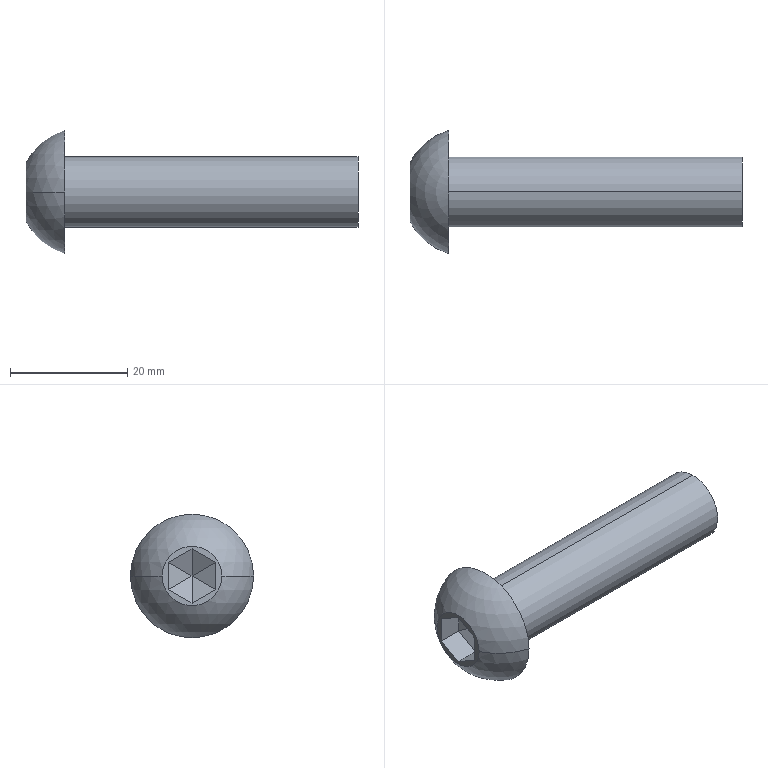Part | SolidWorks | features Cut 2, RevCut 2, Boss 1, Extrusion 1, Fillet 1, LPattern 1 | 1 solid | 19 faces | box 56.6 x 21 x 21 mm | volume 6942 mm3 | plane 15 | sphere 2 | cylinder 2 | commonest cylinder face diameters 12 x2
STEP:
#1=CARTESIAN_POINT('',(6.6,10.5,0.));
#2=VERTEX_POINT('',#1);
#3=CARTESIAN_POINT('',(6.6,-10.5,0.));
#4=VERTEX_POINT('',#3);
#5=CARTESIAN_POINT('',(6.6,0.,0.));
#6=DIRECTION('',(-1.,0.,0.));
#7=DIRECTION('',(0.,0.,1.));
#8=AXIS2_PLACEMENT_3D('',#5,#6,#7);
#9=CIRCLE('',#8,10.5);
#10=EDGE_CURVE('',#2,#4,#9,.T.);
#11=ORIENTED_EDGE('',*,*,#10,.T.);
#12=CARTESIAN_POINT('',(0.,-5.075,0.));
#13=VERTEX_POINT('',#12);
#14=CARTESIAN_POINT('',(9.701,0.,0.));
#15=DIRECTION('',(0.,0.,-1.));
#16=DIRECTION('',(0.,1.,0.));
#17=AXIS2_PLACEMENT_3D('',#14,#15,#16);
#18=CIRCLE('',#17,10.948);
#19=EDGE_CURVE('',#4,#13,#18,.T.);
#20=ORIENTED_EDGE('',*,*,#19,.T.);
#21=CARTESIAN_POINT('',(0.,5.075,0.));
#22=VERTEX_POINT('',#21);
#23=CARTESIAN_POINT('',(0.,0.,0.));
#24=DIRECTION('',(-1.,0.,0.));
#25=DIRECTION('',(0.,0.,1.));
#26=AXIS2_PLACEMENT_3D('',#23,#24,#25);
#27=CIRCLE('',#26,5.075);
#28=EDGE_CURVE('',#22,#13,#27,.T.);
#29=ORIENTED_EDGE('',*,*,#28,.F.);
#30=CARTESIAN_POINT('',(9.701,0.,0.));
#31=DIRECTION('',(0.,0.,1.));
#32=DIRECTION('',(1.,0.,0.));
#33=AXIS2_PLACEMENT_3D('',#30,#31,#32);
#34=CIRCLE('',#33,10.948);
#35=EDGE_CURVE('',#2,#22,#34,.T.);
#36=ORIENTED_EDGE('',*,*,#35,.F.);
#37=EDGE_LOOP('',(#11,#20,#29,#36));
#38=FACE_OUTER_BOUND('',#37,.T.);
#39=CARTESIAN_POINT('',(9.701,0.,0.));
#40=DIRECTION('',(0.,0.,-1.));
#41=DIRECTION('',(0.,1.,0.));
#42=AXIS2_PLACEMENT_3D('',#39,#40,#41);
#43=SPHERICAL_SURFACE('',#42,10.948);
#44=ADVANCED_FACE('',(#38),#43,.T.);
#45=CARTESIAN_POINT('',(56.6,0.,-6.));
#46=VERTEX_POINT('',#45);
#47=CARTESIAN_POINT('',(56.6,0.,6.));
#48=VERTEX_POINT('',#47);
#49=CARTESIAN_POINT('',(56.6,0.,0.));
#50=DIRECTION('',(1.,0.,0.));
#51=DIRECTION('',(0.,0.,-1.));
#52=AXIS2_PLACEMENT_3D('',#49,#50,#51);
#53=CIRCLE('',#52,6.);
#54=EDGE_CURVE('',#46,#48,#53,.T.);
#55=ORIENTED_EDGE('',*,*,#54,.F.);
#56=CARTESIAN_POINT('',(6.6,0.,-6.));
#57=VERTEX_POINT('',#56);
#58=CARTESIAN_POINT('',(56.6,0.,-6.));
#59=DIRECTION('',(-1.,0.,0.));
#60=VECTOR('',#59,1000.);
#61=LINE('',#58,#60);
#62=EDGE_CURVE('',#46,#57,#61,.T.);
#63=ORIENTED_EDGE('',*,*,#62,.T.);
#64=CARTESIAN_POINT('',(6.6,0.,6.));
#65=VERTEX_POINT('',#64);
#66=CARTESIAN_POINT('',(6.6,0.,0.));
#67=DIRECTION('',(1.,0.,0.));
#68=DIRECTION('',(0.,0.,-1.));
#69=AXIS2_PLACEMENT_3D('',#66,#67,#68);
#70=CIRCLE('',#69,6.);
#71=EDGE_CURVE('',#57,#65,#70,.T.);
#72=ORIENTED_EDGE('',*,*,#71,.T.);
#73=CARTESIAN_POINT('',(56.6,0.,6.));
#74=DIRECTION('',(-1.,0.,0.));
#75=VECTOR('',#74,1000.);
#76=LINE('',#73,#75);
#77=EDGE_CURVE('',#48,#65,#76,.T.);
#78=ORIENTED_EDGE('',*,*,#77,.F.);
#79=EDGE_LOOP('',(#55,#63,#72,#78));
#80=FACE_OUTER_BOUND('',#79,.T.);
#81=CARTESIAN_POINT('',(56.6,0.,0.));
#82=DIRECTION('',(-1.,0.,0.));
#83=DIRECTION('',(0.,0.,1.));
#84=AXIS2_PLACEMENT_3D('',#81,#82,#83);
#85=CYLINDRICAL_SURFACE('',#84,6.);
#86=ADVANCED_FACE('',(#80),#85,.T.);
#87=ORIENTED_EDGE('',*,*,#28,.T.);
#88=CARTESIAN_POINT('',(0.,0.,0.));
#89=DIRECTION('',(-1.,0.,0.));
#90=DIRECTION('',(0.,0.,1.));
#91=AXIS2_PLACEMENT_3D('',#88,#89,#90);
#92=CIRCLE('',#91,5.075);
#93=EDGE_CURVE('',#13,#22,#92,.T.);
#94=ORIENTED_EDGE('',*,*,#93,.T.);
#95=EDGE_LOOP('',(#87,#94));
#96=FACE_OUTER_BOUND('',#95,.T.);
#97=CARTESIAN_POINT('',(0.,-4.,-2.309));
#98=VERTEX_POINT('',#97);
#99=CARTESIAN_POINT('',(0.,0.,-4.619));
#100=VERTEX_POINT('',#99);
#101=CARTESIAN_POINT('',(0.,-4.,-2.309));
#102=DIRECTION('',(0.,0.866,-0.5));
#103=VECTOR('',#102,1000.);
#104=LINE('',#101,#103);
#105=EDGE_CURVE('',#98,#100,#104,.T.);
#106=ORIENTED_EDGE('',*,*,#105,.T.);
#107=CARTESIAN_POINT('',(0.,4.,-2.309));
#108=VERTEX_POINT('',#107);
#109=CARTESIAN_POINT('',(0.,0.,-4.619));
#110=DIRECTION('',(0.,0.866,0.5));
#111=VECTOR('',#110,1000.);
#112=LINE('',#109,#111);
#113=EDGE_CURVE('',#100,#108,#112,.T.);
#114=ORIENTED_EDGE('',*,*,#113,.T.);
#115=CARTESIAN_POINT('',(0.,4.,2.309));
#116=VERTEX_POINT('',#115);
#117=CARTESIAN_POINT('',(0.,4.,-2.309));
#118=DIRECTION('',(0.,0.,1.));
#119=VECTOR('',#118,1000.);
#120=LINE('',#117,#119);
#121=EDGE_CURVE('',#108,#116,#120,.T.);
#122=ORIENTED_EDGE('',*,*,#121,.T.);
#123=CARTESIAN_POINT('',(0.,0.,4.619));
#124=VERTEX_POINT('',#123);
#125=CARTESIAN_POINT('',(0.,4.,2.309));
#126=DIRECTION('',(0.,-0.866,0.5));
#127=VECTOR('',#126,1000.);
#128=LINE('',#125,#127);
#129=EDGE_CURVE('',#116,#124,#128,.T.);
#130=ORIENTED_EDGE('',*,*,#129,.T.);
#131=CARTESIAN_POINT('',(0.,-4.,2.309));
#132=VERTEX_POINT('',#131);
#133=CARTESIAN_POINT('',(0.,0.,4.619));
#134=DIRECTION('',(0.,-0.866,-0.5));
#135=VECTOR('',#134,1000.);
#136=LINE('',#133,#135);
#137=EDGE_CURVE('',#124,#132,#136,.T.);
#138=ORIENTED_EDGE('',*,*,#137,.T.);
#139=CARTESIAN_POINT('',(0.,-4.,2.309));
#140=DIRECTION('',(0.,0.,-1.));
#141=VECTOR('',#140,1000.);
#142=LINE('',#139,#141);
#143=EDGE_CURVE('',#132,#98,#142,.T.);
#144=ORIENTED_EDGE('',*,*,#143,.T.);
#145=EDGE_LOOP('',(#106,#114,#122,#130,#138,#144));
#146=FACE_BOUND('',#145,.T.);
#147=CARTESIAN_POINT('',(0.,0.,0.));
#148=DIRECTION('',(1.,0.,0.));
#149=DIRECTION('',(0.,0.,-1.));
#150=AXIS2_PLACEMENT_3D('',#147,#148,#149);
#151=PLANE('',#150);
#152=ADVANCED_FACE('',(#96,#146),#151,.F.);
#153=ORIENTED_EDGE('',*,*,#10,.F.);
#154=CARTESIAN_POINT('',(6.6,0.,0.));
#155=DIRECTION('',(-1.,0.,0.));
#156=DIRECTION('',(0.,0.,1.));
#157=AXIS2_PLACEMENT_3D('',#154,#155,#156);
#158=CIRCLE('',#157,10.5);
#159=EDGE_CURVE('',#4,#2,#158,.T.);
#160=ORIENTED_EDGE('',*,*,#159,.F.);
#161=EDGE_LOOP('',(#153,#160));
#162=FACE_OUTER_BOUND('',#161,.T.);
#163=CARTESIAN_POINT('',(6.6,0.,0.));
#164=DIRECTION('',(1.,0.,0.));
#165=DIRECTION('',(0.,0.,-1.));
#166=AXIS2_PLACEMENT_3D('',#163,#164,#165);
#167=CIRCLE('',#166,6.);
#168=EDGE_CURVE('',#65,#57,#167,.T.);
#169=ORIENTED_EDGE('',*,*,#168,.F.);
#170=ORIENTED_EDGE('',*,*,#71,.F.);
#171=EDGE_LOOP('',(#169,#170));
#172=FACE_BOUND('',#171,.T.);
#173=CARTESIAN_POINT('',(6.6,0.,0.));
#174=DIRECTION('',(1.,0.,0.));
#175=DIRECTION('',(0.,0.,-1.));
#176=AXIS2_PLACEMENT_3D('',#173,#174,#175);
#177=PLANE('',#176);
#178=ADVANCED_FACE('',(#162,#172),#177,.T.);
#179=ORIENTED_EDGE('',*,*,#62,.F.);
#180=CARTESIAN_POINT('',(56.6,0.,0.));
#181=DIRECTION('',(1.,0.,0.));
#182=DIRECTION('',(0.,0.,-1.));
#183=AXIS2_PLACEMENT_3D('',#180,#181,#182);
#184=CIRCLE('',#183,6.);
#185=EDGE_CURVE('',#48,#46,#184,.T.);
#186=ORIENTED_EDGE('',*,*,#185,.F.);
#187=ORIENTED_EDGE('',*,*,#77,.T.);
#188=ORIENTED_EDGE('',*,*,#168,.T.);
#189=EDGE_LOOP('',(#179,#186,#187,#188));
#190=FACE_OUTER_BOUND('',#189,.T.);
#191=CARTESIAN_POINT('',(56.6,0.,0.));
#192=DIRECTION('',(-1.,0.,0.));
#193=DIRECTION('',(0.,0.,1.));
#194=AXIS2_PLACEMENT_3D('',#191,#192,#193);
#195=CYLINDRICAL_SURFACE('',#194,6.);
#196=ADVANCED_FACE('',(#190),#195,.T.);
#197=ORIENTED_EDGE('',*,*,#185,.T.);
#198=ORIENTED_EDGE('',*,*,#54,.T.);
#199=EDGE_LOOP('',(#197,#198));
#200=FACE_OUTER_BOUND('',#199,.T.);
#201=CARTESIAN_POINT('',(56.6,0.,0.));
#202=DIRECTION('',(1.,0.,0.));
#203=DIRECTION('',(0.,0.,-1.));
#204=AXIS2_PLACEMENT_3D('',#201,#202,#203);
#205=PLANE('',#204);
#206=ADVANCED_FACE('',(#200),#205,.T.);
#207=ORIENTED_EDGE('',*,*,#19,.F.);
#208=ORIENTED_EDGE('',*,*,#159,.T.);
#209=ORIENTED_EDGE('',*,*,#35,.T.);
#210=ORIENTED_EDGE('',*,*,#93,.F.);
#211=EDGE_LOOP('',(#207,#208,#209,#210));
#212=FACE_OUTER_BOUND('',#211,.T.);
#213=CARTESIAN_POINT('',(9.701,0.,0.));
#214=DIRECTION('',(0.,0.,-1.));
#215=DIRECTION('',(0.,1.,0.));
#216=AXIS2_PLACEMENT_3D('',#213,#214,#215);
#217=SPHERICAL_SURFACE('',#216,10.948);
#218=ADVANCED_FACE('',(#212),#217,.T.);
#219=ORIENTED_EDGE('',*,*,#105,.F.);
#220=CARTESIAN_POINT('',(4.16,-4.,-2.309));
#221=VERTEX_POINT('',#220);
#222=CARTESIAN_POINT('',(4.16,-4.,-2.309));
#223=DIRECTION('',(-1.,0.,0.));
#224=VECTOR('',#223,1000.);
#225=LINE('',#222,#224);
#226=EDGE_CURVE('',#221,#98,#225,.T.);
#227=ORIENTED_EDGE('',*,*,#226,.F.);
#228=CARTESIAN_POINT('',(4.16,0.,-4.619));
#229=VERTEX_POINT('',#228);
#230=CARTESIAN_POINT('',(4.16,-4.,-2.309));
#231=DIRECTION('',(0.,0.866,-0.5));
#232=VECTOR('',#231,1000.);
#233=LINE('',#230,#232);
#234=EDGE_CURVE('',#221,#229,#233,.T.);
#235=ORIENTED_EDGE('',*,*,#234,.T.);
#236=CARTESIAN_POINT('',(4.16,0.,-4.619));
#237=DIRECTION('',(-1.,0.,0.));
#238=VECTOR('',#237,1000.);
#239=LINE('',#236,#238);
#240=EDGE_CURVE('',#229,#100,#239,.T.);
#241=ORIENTED_EDGE('',*,*,#240,.T.);
#242=EDGE_LOOP('',(#219,#227,#235,#241));
#243=FACE_OUTER_BOUND('',#242,.T.);
#244=CARTESIAN_POINT('',(4.16,-4.,-2.309));
#245=DIRECTION('',(0.,0.5,0.866));
#246=DIRECTION('',(0.,-0.866,0.5));
#247=AXIS2_PLACEMENT_3D('',#244,#245,#246);
#248=PLANE('',#247);
#249=ADVANCED_FACE('',(#243),#248,.T.);
#250=ORIENTED_EDGE('',*,*,#113,.F.);
#251=ORIENTED_EDGE('',*,*,#240,.F.);
#252=CARTESIAN_POINT('',(4.16,4.,-2.309));
#253=VERTEX_POINT('',#252);
#254=CARTESIAN_POINT('',(4.16,0.,-4.619));
#255=DIRECTION('',(0.,0.866,0.5));
#256=VECTOR('',#255,1000.);
#257=LINE('',#254,#256);
#258=EDGE_CURVE('',#229,#253,#257,.T.);
#259=ORIENTED_EDGE('',*,*,#258,.T.);
#260=CARTESIAN_POINT('',(4.16,4.,-2.309));
#261=DIRECTION('',(-1.,0.,0.));
#262=VECTOR('',#261,1000.);
#263=LINE('',#260,#262);
#264=EDGE_CURVE('',#253,#108,#263,.T.);
#265=ORIENTED_EDGE('',*,*,#264,.T.);
#266=EDGE_LOOP('',(#250,#251,#259,#265));
#267=FACE_OUTER_BOUND('',#266,.T.);
#268=CARTESIAN_POINT('',(4.16,0.,-4.619));
#269=DIRECTION('',(0.,-0.5,0.866));
#270=DIRECTION('',(0.,-0.866,-0.5));
#271=AXIS2_PLACEMENT_3D('',#268,#269,#270);
#272=PLANE('',#271);
#273=ADVANCED_FACE('',(#267),#272,.T.);
#274=ORIENTED_EDGE('',*,*,#121,.F.);
#275=ORIENTED_EDGE('',*,*,#264,.F.);
#276=CARTESIAN_POINT('',(4.16,4.,2.309));
#277=VERTEX_POINT('',#276);
#278=CARTESIAN_POINT('',(4.16,4.,-2.309));
#279=DIRECTION('',(0.,0.,1.));
#280=VECTOR('',#279,1000.);
#281=LINE('',#278,#280);
#282=EDGE_CURVE('',#253,#277,#281,.T.);
#283=ORIENTED_EDGE('',*,*,#282,.T.);
#284=CARTESIAN_POINT('',(4.16,4.,2.309));
#285=DIRECTION('',(-1.,0.,0.));
#286=VECTOR('',#285,1000.);
#287=LINE('',#284,#286);
#288=EDGE_CURVE('',#277,#116,#287,.T.);
#289=ORIENTED_EDGE('',*,*,#288,.T.);
#290=EDGE_LOOP('',(#274,#275,#283,#289));
#291=FACE_OUTER_BOUND('',#290,.T.);
#292=CARTESIAN_POINT('',(4.16,4.,-2.309));
#293=DIRECTION('',(0.,-1.,0.));
#294=DIRECTION('',(0.,0.,-1.));
#295=AXIS2_PLACEMENT_3D('',#292,#293,#294);
#296=PLANE('',#295);
#297=ADVANCED_FACE('',(#291),#296,.T.);
#298=ORIENTED_EDGE('',*,*,#129,.F.);
#299=ORIENTED_EDGE('',*,*,#288,.F.);
#300=CARTESIAN_POINT('',(4.16,0.,4.619));
#301=VERTEX_POINT('',#300);
#302=CARTESIAN_POINT('',(4.16,4.,2.309));
#303=DIRECTION('',(0.,-0.866,0.5));
#304=VECTOR('',#303,1000.);
#305=LINE('',#302,#304);
#306=EDGE_CURVE('',#277,#301,#305,.T.);
#307=ORIENTED_EDGE('',*,*,#306,.T.);
#308=CARTESIAN_POINT('',(4.16,0.,4.619));
#309=DIRECTION('',(-1.,0.,0.));
#310=VECTOR('',#309,1000.);
#311=LINE('',#308,#310);
#312=EDGE_CURVE('',#301,#124,#311,.T.);
#313=ORIENTED_EDGE('',*,*,#312,.T.);
#314=EDGE_LOOP('',(#298,#299,#307,#313));
#315=FACE_OUTER_BOUND('',#314,.T.);
#316=CARTESIAN_POINT('',(4.16,4.,2.309));
#317=DIRECTION('',(0.,-0.5,-0.866));
#318=DIRECTION('',(0.,0.866,-0.5));
#319=AXIS2_PLACEMENT_3D('',#316,#317,#318);
#320=PLANE('',#319);
#321=ADVANCED_FACE('',(#315),#320,.T.);
#322=ORIENTED_EDGE('',*,*,#137,.F.);
#323=ORIENTED_EDGE('',*,*,#312,.F.);
#324=CARTESIAN_POINT('',(4.16,-4.,2.309));
#325=VERTEX_POINT('',#324);
#326=CARTESIAN_POINT('',(4.16,0.,4.619));
#327=DIRECTION('',(0.,-0.866,-0.5));
#328=VECTOR('',#327,1000.);
#329=LINE('',#326,#328);
#330=EDGE_CURVE('',#301,#325,#329,.T.);
#331=ORIENTED_EDGE('',*,*,#330,.T.);
#332=CARTESIAN_POINT('',(4.16,-4.,2.309));
#333=DIRECTION('',(-1.,0.,0.));
#334=VECTOR('',#333,1000.);
#335=LINE('',#332,#334);
#336=EDGE_CURVE('',#325,#132,#335,.T.);
#337=ORIENTED_EDGE('',*,*,#336,.T.);
#338=EDGE_LOOP('',(#322,#323,#331,#337));
#339=FACE_OUTER_BOUND('',#338,.T.);
#340=CARTESIAN_POINT('',(4.16,0.,4.619));
#341=DIRECTION('',(0.,0.5,-0.866));
#342=DIRECTION('',(0.,0.866,0.5));
#343=AXIS2_PLACEMENT_3D('',#340,#341,#342);
#344=PLANE('',#343);
#345=ADVANCED_FACE('',(#339),#344,.T.);
#346=ORIENTED_EDGE('',*,*,#143,.F.);
#347=ORIENTED_EDGE('',*,*,#336,.F.);
#348=CARTESIAN_POINT('',(4.16,-4.,2.309));
#349=DIRECTION('',(0.,0.,-1.));
#350=VECTOR('',#349,1000.);
#351=LINE('',#348,#350);
#352=EDGE_CURVE('',#325,#221,#351,.T.);
#353=ORIENTED_EDGE('',*,*,#352,.T.);
#354=ORIENTED_EDGE('',*,*,#226,.T.);
#355=EDGE_LOOP('',(#346,#347,#353,#354));
#356=FACE_OUTER_BOUND('',#355,.T.);
#357=CARTESIAN_POINT('',(4.16,-4.,2.309));
#358=DIRECTION('',(0.,1.,0.));
#359=DIRECTION('',(0.,0.,1.));
#360=AXIS2_PLACEMENT_3D('',#357,#358,#359);
#361=PLANE('',#360);
#362=ADVANCED_FACE('',(#356),#361,.T.);
#363=ORIENTED_EDGE('',*,*,#330,.F.);
#364=CARTESIAN_POINT('',(6.469,0.,0.));
#365=VERTEX_POINT('',#364);
#366=CARTESIAN_POINT('',(4.16,0.,4.619));
#367=DIRECTION('',(-0.4472,0.,0.8944));
#368=VECTOR('',#367,1000.);
#369=LINE('',#366,#368);
#370=EDGE_CURVE('',#365,#301,#369,.T.);
#371=ORIENTED_EDGE('',*,*,#370,.F.);
#372=CARTESIAN_POINT('',(4.16,-4.,2.309));
#373=DIRECTION('',(-0.4472,-0.7746,0.4472));
#374=VECTOR('',#373,1000.);
#375=LINE('',#372,#374);
#376=EDGE_CURVE('',#365,#325,#375,.T.);
#377=ORIENTED_EDGE('',*,*,#376,.T.);
#378=EDGE_LOOP('',(#363,#371,#377));
#379=FACE_OUTER_BOUND('',#378,.T.);
#380=CARTESIAN_POINT('',(4.16,0.,4.619));
#381=DIRECTION('',(0.866,-0.25,0.433));
#382=DIRECTION('',(0.4472,0.,-0.8944));
#383=AXIS2_PLACEMENT_3D('',#380,#381,#382);
#384=PLANE('',#383);
#385=ADVANCED_FACE('',(#379),#384,.F.);
#386=ORIENTED_EDGE('',*,*,#352,.F.);
#387=ORIENTED_EDGE('',*,*,#376,.F.);
#388=CARTESIAN_POINT('',(4.16,-4.,-2.309));
#389=DIRECTION('',(-0.4472,-0.7746,-0.4472));
#390=VECTOR('',#389,1000.);
#391=LINE('',#388,#390);
#392=EDGE_CURVE('',#365,#221,#391,.T.);
#393=ORIENTED_EDGE('',*,*,#392,.T.);
#394=EDGE_LOOP('',(#386,#387,#393));
#395=FACE_OUTER_BOUND('',#394,.T.);
#396=CARTESIAN_POINT('',(4.16,-4.,2.309));
#397=DIRECTION('',(0.866,-0.5,0.));
#398=DIRECTION('',(0.5,0.866,0.));
#399=AXIS2_PLACEMENT_3D('',#396,#397,#398);
#400=PLANE('',#399);
#401=ADVANCED_FACE('',(#395),#400,.F.);
#402=ORIENTED_EDGE('',*,*,#234,.F.);
#403=ORIENTED_EDGE('',*,*,#392,.F.);
#404=CARTESIAN_POINT('',(4.16,0.,-4.619));
#405=DIRECTION('',(-0.4472,0.,-0.8944));
#406=VECTOR('',#405,1000.);
#407=LINE('',#404,#406);
#408=EDGE_CURVE('',#365,#229,#407,.T.);
#409=ORIENTED_EDGE('',*,*,#408,.T.);
#410=EDGE_LOOP('',(#402,#403,#409));
#411=FACE_OUTER_BOUND('',#410,.T.);
#412=CARTESIAN_POINT('',(4.16,-4.,-2.309));
#413=DIRECTION('',(0.866,-0.25,-0.433));
#414=DIRECTION('',(-0.4472,0.,-0.8944));
#415=AXIS2_PLACEMENT_3D('',#412,#413,#414);
#416=PLANE('',#415);
#417=ADVANCED_FACE('',(#411),#416,.F.);
#418=ORIENTED_EDGE('',*,*,#258,.F.);
#419=ORIENTED_EDGE('',*,*,#408,.F.);
#420=CARTESIAN_POINT('',(4.16,4.,-2.309));
#421=DIRECTION('',(-0.4472,0.7746,-0.4472));
#422=VECTOR('',#421,1000.);
#423=LINE('',#420,#422);
#424=EDGE_CURVE('',#365,#253,#423,.T.);
#425=ORIENTED_EDGE('',*,*,#424,.T.);
#426=EDGE_LOOP('',(#418,#419,#425));
#427=FACE_OUTER_BOUND('',#426,.T.);
#428=CARTESIAN_POINT('',(4.16,0.,-4.619));
#429=DIRECTION('',(0.866,0.25,-0.433));
#430=DIRECTION('',(-0.4472,0.,-0.8944));
#431=AXIS2_PLACEMENT_3D('',#428,#429,#430);
#432=PLANE('',#431);
#433=ADVANCED_FACE('',(#427),#432,.F.);
#434=ORIENTED_EDGE('',*,*,#282,.F.);
#435=ORIENTED_EDGE('',*,*,#424,.F.);
#436=CARTESIAN_POINT('',(4.16,4.,2.309));
#437=DIRECTION('',(-0.4472,0.7746,0.4472));
#438=VECTOR('',#437,1000.);
#439=LINE('',#436,#438);
#440=EDGE_CURVE('',#365,#277,#439,.T.);
#441=ORIENTED_EDGE('',*,*,#440,.T.);
#442=EDGE_LOOP('',(#434,#435,#441));
#443=FACE_OUTER_BOUND('',#442,.T.);
#444=CARTESIAN_POINT('',(4.16,4.,-2.309));
#445=DIRECTION('',(0.866,0.5,0.));
#446=DIRECTION('',(-0.5,0.866,0.));
#447=AXIS2_PLACEMENT_3D('',#444,#445,#446);
#448=PLANE('',#447);
#449=ADVANCED_FACE('',(#443),#448,.F.);
#450=ORIENTED_EDGE('',*,*,#306,.F.);
#451=ORIENTED_EDGE('',*,*,#440,.F.);
#452=ORIENTED_EDGE('',*,*,#370,.T.);
#453=EDGE_LOOP('',(#450,#451,#452));
#454=FACE_OUTER_BOUND('',#453,.T.);
#455=CARTESIAN_POINT('',(4.16,4.,2.309));
#456=DIRECTION('',(0.866,0.25,0.433));
#457=DIRECTION('',(0.4472,0.,-0.8944));
#458=AXIS2_PLACEMENT_3D('',#455,#456,#457);
#459=PLANE('',#458);
#460=ADVANCED_FACE('',(#454),#459,.F.);
#461=CLOSED_SHELL('',(#44,#86,#152,#178,#196,#206,#218,#249,#273,#297,#321,#345,#362,#385,#401,#417,#433,#449,#460));
#462=MANIFOLD_SOLID_BREP('',#461);
#463=CARTESIAN_POINT('',(0.,0.,0.));
#464=DIRECTION('',(0.,0.,1.));
#465=DIRECTION('',(1.,0.,0.));
#466=AXIS2_PLACEMENT_3D('',#463,#464,#465);
#467=(LENGTH_UNIT()NAMED_UNIT(*)SI_UNIT(.MILLI.,.METRE.));
#468=UNCERTAINTY_MEASURE_WITH_UNIT(LENGTH_MEASURE(0.00001),#467,'','');
#469=(NAMED_UNIT(*)PLANE_ANGLE_UNIT()SI_UNIT($,.RADIAN.));
#470=(NAMED_UNIT(*)SI_UNIT($,.STERADIAN.)SOLID_ANGLE_UNIT());
#471=(GEOMETRIC_REPRESENTATION_CONTEXT(3)GLOBAL_UNCERTAINTY_ASSIGNED_CONTEXT((#468))GLOBAL_UNIT_ASSIGNED_CONTEXT((#467,#469,#470))REPRESENTATION_CONTEXT('',''));
#472=ADVANCED_BREP_SHAPE_REPRESENTATION('',(#462,#466),#471);